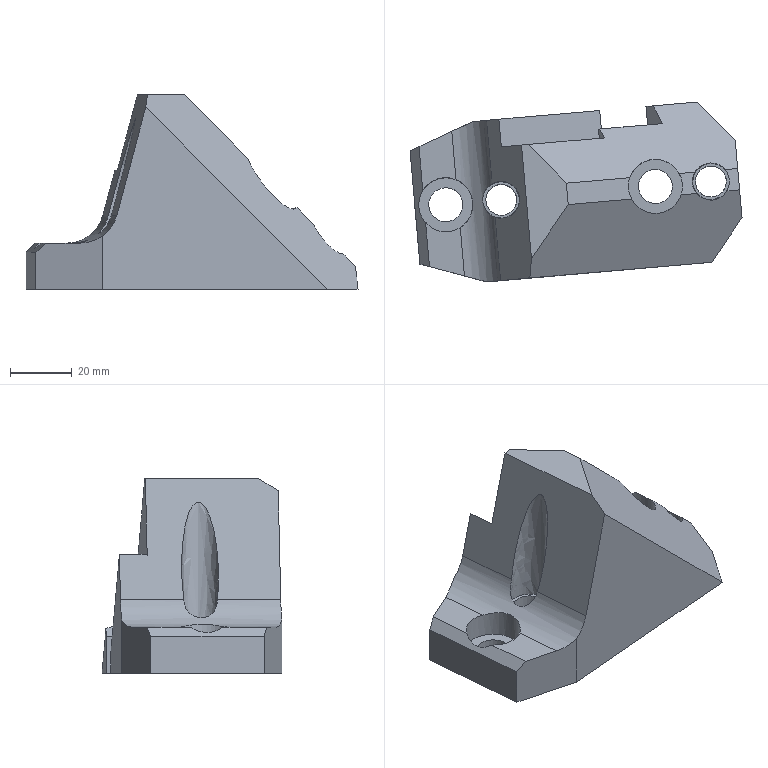Part | NX | features solid 2 | 1 solid | 40 faces | box 107.293 x 58.165 x 63 mm | volume 136956 mm3 | plane 31 | cylinder 7 | spline 2 | commonest cylinder face diameters 10 x2 11 x2 17.5 x2 24 x1
STEP:
#1=CARTESIAN_POINT('',(-404.06,16.31,45.514));
#2=VERTEX_POINT('',#1);
#3=CARTESIAN_POINT('',(-413.818,15.456,55.309));
#4=VERTEX_POINT('',#3);
#5=CARTESIAN_POINT('',(-404.06,16.31,45.514));
#6=CARTESIAN_POINT('',(-404.91,17.317,45.393));
#7=CARTESIAN_POINT('',(-407.23,18.575,46.406));
#8=CARTESIAN_POINT('',(-410.106,18.429,49.198));
#9=CARTESIAN_POINT('',(-412.325,17.358,52.216));
#10=CARTESIAN_POINT('',(-413.406,16.165,54.29));
#11=CARTESIAN_POINT('',(-413.818,15.456,55.309));
#12=B_SPLINE_CURVE_WITH_KNOTS('',3,(#5,#6,#7,#8,#9,#10,#11),.UNSPECIFIED.,.F.,.F.,(4,1,1,1,4),(-0.007434,-0.003558,0.0003178,0.004194,0.00807),.UNSPECIFIED.);
#13=EDGE_CURVE('',#2,#4,#12,.T.);
#14=ORIENTED_EDGE('',*,*,#13,.F.);
#15=CARTESIAN_POINT('',(-399.975,16.667,41.413));
#16=VERTEX_POINT('',#15);
#17=CARTESIAN_POINT('',(-490.277,8.767,132.06));
#18=DIRECTION('',(0.7044,0.06163,-0.7071));
#19=VECTOR('',#18,1000.);
#20=LINE('',#17,#19);
#21=EDGE_CURVE('',#2,#16,#20,.T.);
#22=ORIENTED_EDGE('',*,*,#21,.T.);
#23=CARTESIAN_POINT('',(-400.766,25.712,34.));
#24=VERTEX_POINT('',#23);
#25=CARTESIAN_POINT('',(-397.614,-10.317,63.53));
#26=DIRECTION('',(0.06751,-0.7716,0.6325));
#27=VECTOR('',#26,1000.);
#28=LINE('',#25,#27);
#29=EDGE_CURVE('',#24,#16,#28,.T.);
#30=ORIENTED_EDGE('',*,*,#29,.F.);
#31=CARTESIAN_POINT('',(-412.885,38.16,34.));
#32=VERTEX_POINT('',#31);
#33=CARTESIAN_POINT('',(-451.45,77.774,34.));
#34=DIRECTION('',(-0.6976,0.7165,0.));
#35=VECTOR('',#34,1000.);
#36=LINE('',#33,#35);
#37=EDGE_CURVE('',#24,#32,#36,.T.);
#38=ORIENTED_EDGE('',*,*,#37,.T.);
#39=CARTESIAN_POINT('',(-427.238,36.904,48.408));
#40=VERTEX_POINT('',#39);
#41=CARTESIAN_POINT('',(-501.407,30.415,122.86));
#42=DIRECTION('',(0.7044,0.06163,-0.7071));
#43=VECTOR('',#42,1000.);
#44=LINE('',#41,#43);
#45=EDGE_CURVE('',#40,#32,#44,.T.);
#46=ORIENTED_EDGE('',*,*,#45,.F.);
#47=CARTESIAN_POINT('',(-424.275,31.141,50.857));
#48=VERTEX_POINT('',#47);
#49=CARTESIAN_POINT('',(-426.8,36.054,48.769));
#50=DIRECTION('',(0.4277,-0.8319,0.3536));
#51=VECTOR('',#50,1000.);
#52=LINE('',#49,#51);
#53=EDGE_CURVE('',#40,#48,#52,.T.);
#54=ORIENTED_EDGE('',*,*,#53,.T.);
#55=CARTESIAN_POINT('',(-444.558,29.366,71.219));
#56=VERTEX_POINT('',#55);
#57=CARTESIAN_POINT('',(-498.443,24.652,125.31));
#58=DIRECTION('',(-0.7044,-0.06163,0.7071));
#59=VECTOR('',#58,1000.);
#60=LINE('',#57,#59);
#61=EDGE_CURVE('',#48,#56,#60,.T.);
#62=ORIENTED_EDGE('',*,*,#61,.T.);
#63=CARTESIAN_POINT('',(-443.077,26.484,72.444));
#64=VERTEX_POINT('',#63);
#65=CARTESIAN_POINT('',(-447.084,34.279,69.131));
#66=DIRECTION('',(0.4277,-0.8319,0.3536));
#67=VECTOR('',#66,1000.);
#68=LINE('',#65,#67);
#69=EDGE_CURVE('',#56,#64,#68,.T.);
#70=ORIENTED_EDGE('',*,*,#69,.T.);
#71=CARTESIAN_POINT('',(-467.54,24.344,97.));
#72=VERTEX_POINT('',#71);
#73=CARTESIAN_POINT('',(-496.962,21.77,126.534));
#74=DIRECTION('',(0.7044,0.06163,-0.7071));
#75=VECTOR('',#74,1000.);
#76=LINE('',#73,#75);
#77=EDGE_CURVE('',#72,#64,#76,.T.);
#78=ORIENTED_EDGE('',*,*,#77,.F.);
#79=CARTESIAN_POINT('',(-455.35,11.823,97.));
#80=VERTEX_POINT('',#79);
#81=CARTESIAN_POINT('',(-486.416,43.733,97.));
#82=DIRECTION('',(-0.6976,0.7165,0.));
#83=VECTOR('',#82,1000.);
#84=LINE('',#81,#83);
#85=EDGE_CURVE('',#80,#72,#84,.T.);
#86=ORIENTED_EDGE('',*,*,#85,.F.);
#87=CARTESIAN_POINT('',(-434.875,13.614,76.447));
#88=VERTEX_POINT('',#87);
#89=CARTESIAN_POINT('',(-490.277,8.767,132.06));
#90=DIRECTION('',(0.7044,0.06163,-0.7071));
#91=VECTOR('',#90,1000.);
#92=LINE('',#89,#91);
#93=EDGE_CURVE('',#80,#88,#92,.T.);
#94=ORIENTED_EDGE('',*,*,#93,.T.);
#95=CARTESIAN_POINT('',(-418.866,15.015,60.376));
#96=VERTEX_POINT('',#95);
#97=CARTESIAN_POINT('',(-426.569,10.863,71.24));
#98=DIRECTION('',(-0.5665,-0.5515,-0.6124));
#99=DIRECTION('',(0.4388,0.4272,-0.7906));
#100=AXIS2_PLACEMENT_3D('',#97,#98,#99);
#101=ELLIPSE('',#100,14.289,8.75);
#102=EDGE_CURVE('',#96,#88,#101,.F.);
#103=ORIENTED_EDGE('',*,*,#102,.F.);
#104=CARTESIAN_POINT('',(-490.277,8.767,132.06));
#105=DIRECTION('',(0.7044,0.06163,-0.7071));
#106=VECTOR('',#105,1000.);
#107=LINE('',#104,#106);
#108=EDGE_CURVE('',#96,#4,#107,.T.);
#109=ORIENTED_EDGE('',*,*,#108,.T.);
#110=EDGE_LOOP('',(#14,#22,#30,#38,#46,#54,#62,#70,#78,#86,#94,#103,#109));
#111=FACE_BOUND('',#110,.T.);
#112=CARTESIAN_POINT('',(-500.969,29.565,123.222));
#113=DIRECTION('',(-0.5665,-0.5515,-0.6124));
#114=DIRECTION('',(-0.7044,-0.06163,0.7071));
#115=AXIS2_PLACEMENT_3D('',#112,#113,#114);
#116=PLANE('',#115);
#117=ADVANCED_FACE('',(#111),#116,.F.);
#118=CARTESIAN_POINT('',(-403.457,9.408,45.514));
#119=VERTEX_POINT('',#118);
#120=CARTESIAN_POINT('',(-399.371,9.766,41.413));
#121=VERTEX_POINT('',#120);
#122=CARTESIAN_POINT('',(-489.673,1.865,132.06));
#123=DIRECTION('',(0.7044,0.06163,-0.7071));
#124=VECTOR('',#123,1000.);
#125=LINE('',#122,#124);
#126=EDGE_CURVE('',#119,#121,#125,.T.);
#127=ORIENTED_EDGE('',*,*,#126,.F.);
#128=CARTESIAN_POINT('',(-413.214,8.555,55.309));
#129=VERTEX_POINT('',#128);
#130=CARTESIAN_POINT('',(-413.214,8.555,55.309));
#131=CARTESIAN_POINT('',(-412.685,7.928,54.289));
#132=CARTESIAN_POINT('',(-411.436,6.953,52.248));
#133=CARTESIAN_POINT('',(-409.038,6.268,49.191));
#134=CARTESIAN_POINT('',(-406.185,6.627,46.407));
#135=CARTESIAN_POINT('',(-404.117,8.271,45.394));
#136=CARTESIAN_POINT('',(-403.457,9.408,45.514));
#137=B_SPLINE_CURVE_WITH_KNOTS('',3,(#130,#131,#132,#133,#134,#135,#136),.UNSPECIFIED.,.F.,.F.,(4,1,1,1,4),(0.,0.003871,0.007742,0.01161,0.01548),.UNSPECIFIED.);
#138=EDGE_CURVE('',#129,#119,#137,.T.);
#139=ORIENTED_EDGE('',*,*,#138,.F.);
#140=CARTESIAN_POINT('',(-418.262,8.113,60.376));
#141=VERTEX_POINT('',#140);
#142=CARTESIAN_POINT('',(-489.673,1.865,132.06));
#143=DIRECTION('',(0.7044,0.06163,-0.7071));
#144=VECTOR('',#143,1000.);
#145=LINE('',#142,#144);
#146=EDGE_CURVE('',#141,#129,#145,.T.);
#147=ORIENTED_EDGE('',*,*,#146,.F.);
#148=CARTESIAN_POINT('',(-434.271,6.712,76.447));
#149=VERTEX_POINT('',#148);
#150=CARTESIAN_POINT('',(-426.569,10.863,71.24));
#151=DIRECTION('',(-0.6536,0.4447,-0.6124));
#152=DIRECTION('',(0.5063,-0.3445,-0.7906));
#153=AXIS2_PLACEMENT_3D('',#150,#151,#152);
#154=ELLIPSE('',#153,14.289,8.75);
#155=EDGE_CURVE('',#149,#141,#154,.F.);
#156=ORIENTED_EDGE('',*,*,#155,.F.);
#157=CARTESIAN_POINT('',(-454.746,4.921,97.));
#158=VERTEX_POINT('',#157);
#159=CARTESIAN_POINT('',(-489.673,1.865,132.06));
#160=DIRECTION('',(0.7044,0.06163,-0.7071));
#161=VECTOR('',#160,1000.);
#162=LINE('',#159,#161);
#163=EDGE_CURVE('',#158,#149,#162,.T.);
#164=ORIENTED_EDGE('',*,*,#163,.F.);
#165=CARTESIAN_POINT('',(-466.613,-12.52,97.));
#166=VERTEX_POINT('',#165);
#167=CARTESIAN_POINT('',(-467.532,-13.87,97.));
#168=DIRECTION('',(0.5625,0.8268,0.));
#169=VECTOR('',#168,1000.);
#170=LINE('',#167,#169);
#171=EDGE_CURVE('',#166,#158,#170,.T.);
#172=ORIENTED_EDGE('',*,*,#171,.F.);
#173=CARTESIAN_POINT('',(-467.138,-18.785,93.01));
#174=VERTEX_POINT('',#173);
#175=CARTESIAN_POINT('',(-464.592,11.602,112.36));
#176=DIRECTION('',(0.0705,0.8414,0.5358));
#177=VECTOR('',#176,1000.);
#178=LINE('',#175,#177);
#179=EDGE_CURVE('',#174,#166,#178,.T.);
#180=ORIENTED_EDGE('',*,*,#179,.F.);
#181=CARTESIAN_POINT('',(-408.352,-13.642,34.));
#182=VERTEX_POINT('',#181);
#183=CARTESIAN_POINT('',(-496.874,-21.387,122.86));
#184=DIRECTION('',(0.7044,0.06163,-0.7071));
#185=VECTOR('',#184,1000.);
#186=LINE('',#183,#185);
#187=EDGE_CURVE('',#174,#182,#186,.T.);
#188=ORIENTED_EDGE('',*,*,#187,.T.);
#189=CARTESIAN_POINT('',(-398.58,0.7211,34.));
#190=VERTEX_POINT('',#189);
#191=CARTESIAN_POINT('',(-427.185,-41.321,34.));
#192=DIRECTION('',(0.5625,0.8268,0.));
#193=VECTOR('',#192,1000.);
#194=LINE('',#191,#193);
#195=EDGE_CURVE('',#182,#190,#194,.T.);
#196=ORIENTED_EDGE('',*,*,#195,.T.);
#197=CARTESIAN_POINT('',(-403.204,53.577,77.322));
#198=DIRECTION('',(0.06751,-0.7716,-0.6325));
#199=VECTOR('',#198,1000.);
#200=LINE('',#197,#199);
#201=EDGE_CURVE('',#121,#190,#200,.T.);
#202=ORIENTED_EDGE('',*,*,#201,.F.);
#203=EDGE_LOOP('',(#127,#139,#147,#156,#164,#172,#180,#188,#196,#202));
#204=FACE_BOUND('',#203,.T.);
#205=CARTESIAN_POINT('',(-489.845,1.312,131.842));
#206=DIRECTION('',(-0.6536,0.4447,-0.6124));
#207=DIRECTION('',(-0.7044,-0.06163,0.7071));
#208=AXIS2_PLACEMENT_3D('',#205,#206,#207);
#209=PLANE('',#208);
#210=ADVANCED_FACE('',(#204),#209,.F.);
#211=CARTESIAN_POINT('',(-403.457,9.408,45.514));
#212=CARTESIAN_POINT('',(-402.887,10.388,44.862));
#213=CARTESIAN_POINT('',(-402.211,12.984,43.962));
#214=CARTESIAN_POINT('',(-403.328,15.443,44.861));
#215=CARTESIAN_POINT('',(-404.06,16.31,45.514));
#216=B_SPLINE_CURVE_WITH_KNOTS('',3,(#211,#212,#213,#214,#215),.UNSPECIFIED.,.F.,.F.,(4,1,4),(0.,0.003881,0.007763),.UNSPECIFIED.);
#217=EDGE_CURVE('',#119,#2,#216,.T.);
#218=ORIENTED_EDGE('',*,*,#217,.F.);
#219=ORIENTED_EDGE('',*,*,#126,.T.);
#220=CARTESIAN_POINT('',(-399.371,9.766,41.413));
#221=DIRECTION('',(0.08716,-0.9962,0.));
#222=VECTOR('',#221,1000.);
#223=LINE('',#220,#222);
#224=EDGE_CURVE('',#16,#121,#223,.T.);
#225=ORIENTED_EDGE('',*,*,#224,.F.);
#226=ORIENTED_EDGE('',*,*,#21,.F.);
#227=EDGE_LOOP('',(#218,#219,#225,#226));
#228=FACE_BOUND('',#227,.T.);
#229=CARTESIAN_POINT('',(-489.673,1.865,132.06));
#230=DIRECTION('',(-0.7044,-0.06163,-0.7071));
#231=DIRECTION('',(-0.7044,-0.06163,0.7071));
#232=AXIS2_PLACEMENT_3D('',#229,#230,#231);
#233=PLANE('',#232);
#234=ADVANCED_FACE('',(#228),#233,.F.);
#235=CARTESIAN_POINT('',(-476.512,-19.605,57.892));
#236=VERTEX_POINT('',#235);
#237=CARTESIAN_POINT('',(-478.299,0.8249,57.892));
#238=VERTEX_POINT('',#237);
#239=CARTESIAN_POINT('',(-476.512,-19.605,57.892));
#240=DIRECTION('',(-0.08716,0.9962,0.));
#241=VECTOR('',#240,1000.);
#242=LINE('',#239,#241);
#243=EDGE_CURVE('',#236,#238,#242,.T.);
#244=ORIENTED_EDGE('',*,*,#243,.T.);
#245=CARTESIAN_POINT('',(-479.257,11.767,57.892));
#246=VERTEX_POINT('',#245);
#247=CARTESIAN_POINT('',(-478.299,0.8249,57.892));
#248=CARTESIAN_POINT('',(-478.516,0.8982,57.109));
#249=CARTESIAN_POINT('',(-479.104,1.119,55.621));
#250=CARTESIAN_POINT('',(-480.41,1.933,53.674));
#251=CARTESIAN_POINT('',(-481.783,3.581,52.36));
#252=CARTESIAN_POINT('',(-482.532,5.948,51.903));
#253=CARTESIAN_POINT('',(-482.215,8.435,52.352));
#254=CARTESIAN_POINT('',(-481.151,10.297,53.663));
#255=CARTESIAN_POINT('',(-480.008,11.331,55.597));
#256=CARTESIAN_POINT('',(-479.458,11.656,57.107));
#257=CARTESIAN_POINT('',(-479.257,11.767,57.892));
#258=B_SPLINE_CURVE_WITH_KNOTS('',3,(#247,#248,#249,#250,#251,#252,#253,#254,#255,#256,#257),.UNSPECIFIED.,.F.,.F.,(4,1,1,1,1,1,1,1,4),(0.,0.002417,0.004835,0.007252,0.009669,0.01209,0.0145,0.01692,0.01934),.UNSPECIFIED.);
#259=EDGE_CURVE('',#238,#246,#258,.T.);
#260=ORIENTED_EDGE('',*,*,#259,.T.);
#261=CARTESIAN_POINT('',(-481.044,32.197,57.892));
#262=VERTEX_POINT('',#261);
#263=CARTESIAN_POINT('',(-476.512,-19.605,57.892));
#264=DIRECTION('',(-0.08716,0.9962,0.));
#265=VECTOR('',#264,1000.);
#266=LINE('',#263,#265);
#267=EDGE_CURVE('',#246,#262,#266,.T.);
#268=ORIENTED_EDGE('',*,*,#267,.T.);
#269=CARTESIAN_POINT('',(-485.618,31.797,51.251));
#270=VERTEX_POINT('',#269);
#271=CARTESIAN_POINT('',(-492.591,31.187,60.998));
#272=DIRECTION('',(0.08716,-0.9962,0.));
#273=DIRECTION('',(0.9962,0.08716,0.));
#274=AXIS2_PLACEMENT_3D('',#271,#272,#273);
#275=CIRCLE('',#274,12.);
#276=EDGE_CURVE('',#270,#262,#275,.T.);
#277=ORIENTED_EDGE('',*,*,#276,.F.);
#278=CARTESIAN_POINT('',(-492.369,28.648,48.998));
#279=VERTEX_POINT('',#278);
#280=CARTESIAN_POINT('',(-492.369,28.648,60.998));
#281=DIRECTION('',(0.4226,-0.9063,0.));
#282=DIRECTION('',(0.9063,0.4226,0.));
#283=AXIS2_PLACEMENT_3D('',#280,#281,#282);
#284=ELLIPSE('',#283,12.77,12.);
#285=EDGE_CURVE('',#279,#270,#284,.T.);
#286=ORIENTED_EDGE('',*,*,#285,.F.);
#287=CARTESIAN_POINT('',(-491.003,13.038,48.998));
#288=VERTEX_POINT('',#287);
#289=CARTESIAN_POINT('',(-488.059,-20.616,48.998));
#290=DIRECTION('',(-0.08716,0.9962,0.));
#291=VECTOR('',#290,1000.);
#292=LINE('',#289,#291);
#293=EDGE_CURVE('',#288,#279,#292,.T.);
#294=ORIENTED_EDGE('',*,*,#293,.F.);
#295=CARTESIAN_POINT('',(-489.647,-2.467,48.998));
#296=VERTEX_POINT('',#295);
#297=CARTESIAN_POINT('',(-491.003,13.038,48.998));
#298=CARTESIAN_POINT('',(-489.499,12.424,48.998));
#299=CARTESIAN_POINT('',(-486.924,10.407,49.531));
#300=CARTESIAN_POINT('',(-485.14,5.744,50.201));
#301=CARTESIAN_POINT('',(-486.079,0.845,49.533));
#302=CARTESIAN_POINT('',(-488.272,-1.601,48.998));
#303=CARTESIAN_POINT('',(-489.647,-2.467,48.998));
#304=B_SPLINE_CURVE_WITH_KNOTS('',3,(#297,#298,#299,#300,#301,#302,#303),.UNSPECIFIED.,.F.,.F.,(4,1,1,1,4),(0.,0.004797,0.009594,0.01439,0.01919),.UNSPECIFIED.);
#305=EDGE_CURVE('',#288,#296,#304,.T.);
#306=ORIENTED_EDGE('',*,*,#305,.T.);
#307=CARTESIAN_POINT('',(-488.281,-18.077,48.998));
#308=VERTEX_POINT('',#307);
#309=CARTESIAN_POINT('',(-488.059,-20.616,48.998));
#310=DIRECTION('',(-0.08716,0.9962,0.));
#311=VECTOR('',#310,1000.);
#312=LINE('',#309,#311);
#313=EDGE_CURVE('',#308,#296,#312,.T.);
#314=ORIENTED_EDGE('',*,*,#313,.F.);
#315=CARTESIAN_POINT('',(-481.086,-20.005,51.251));
#316=VERTEX_POINT('',#315);
#317=CARTESIAN_POINT('',(-488.281,-18.077,60.998));
#318=DIRECTION('',(-0.2588,-0.9659,0.));
#319=DIRECTION('',(-0.9659,0.2588,0.));
#320=AXIS2_PLACEMENT_3D('',#317,#318,#319);
#321=ELLIPSE('',#320,12.77,12.);
#322=EDGE_CURVE('',#308,#316,#321,.T.);
#323=ORIENTED_EDGE('',*,*,#322,.T.);
#324=CARTESIAN_POINT('',(-488.059,-20.616,60.998));
#325=DIRECTION('',(0.08716,-0.9962,0.));
#326=DIRECTION('',(0.9962,0.08716,0.));
#327=AXIS2_PLACEMENT_3D('',#324,#325,#326);
#328=CIRCLE('',#327,12.);
#329=EDGE_CURVE('',#316,#236,#328,.T.);
#330=ORIENTED_EDGE('',*,*,#329,.T.);
#331=EDGE_LOOP('',(#244,#260,#268,#277,#286,#294,#306,#314,#323,#330));
#332=FACE_BOUND('',#331,.T.);
#333=CARTESIAN_POINT('',(-488.059,-20.616,60.998));
#334=DIRECTION('',(-0.08716,0.9962,0.));
#335=DIRECTION('',(0.,0.,1.));
#336=AXIS2_PLACEMENT_3D('',#333,#334,#335);
#337=CYLINDRICAL_SURFACE('',#336,12.);
#338=ADVANCED_FACE('',(#332),#337,.F.);
#339=ORIENTED_EDGE('',*,*,#267,.F.);
#340=CARTESIAN_POINT('',(-479.257,11.767,57.892));
#341=CARTESIAN_POINT('',(-478.55,12.153,60.646));
#342=CARTESIAN_POINT('',(-477.466,12.487,64.785));
#343=CARTESIAN_POINT('',(-475.979,12.526,70.325));
#344=CARTESIAN_POINT('',(-474.849,12.343,74.467));
#345=CARTESIAN_POINT('',(-473.705,11.924,78.582));
#346=CARTESIAN_POINT('',(-472.736,11.321,81.991));
#347=CARTESIAN_POINT('',(-471.957,10.591,84.648));
#348=CARTESIAN_POINT('',(-471.37,9.857,86.591));
#349=CARTESIAN_POINT('',(-470.888,8.997,88.106));
#350=CARTESIAN_POINT('',(-470.535,7.975,89.085));
#351=CARTESIAN_POINT('',(-470.354,6.887,89.402));
#352=CARTESIAN_POINT('',(-470.393,5.853,88.921));
#353=CARTESIAN_POINT('',(-470.583,4.853,87.892));
#354=CARTESIAN_POINT('',(-470.917,3.963,86.359));
#355=CARTESIAN_POINT('',(-471.368,3.169,84.423));
#356=CARTESIAN_POINT('',(-472.012,2.337,81.76));
#357=CARTESIAN_POINT('',(-472.85,1.604,78.405));
#358=CARTESIAN_POINT('',(-473.893,1.008,74.333));
#359=CARTESIAN_POINT('',(-474.965,0.64,70.228));
#360=CARTESIAN_POINT('',(-476.425,0.4275,64.73));
#361=CARTESIAN_POINT('',(-477.542,0.569,60.625));
#362=CARTESIAN_POINT('',(-478.299,0.8249,57.892));
#363=B_SPLINE_CURVE_WITH_KNOTS('',3,(#340,#341,#342,#343,#344,#345,#346,#347,#348,#349,#350,#351,#352,#353,#354,#355,#356,#357,#358,#359,#360,#361,#362),.UNSPECIFIED.,.F.,.F.,(4,1,1,1,1,1,1,1,1,1,1,1,1,1,1,1,1,1,1,1,4),(0.,0.008585,0.01288,0.01717,0.02146,0.02575,0.0279,0.03005,0.03219,0.03327,0.03434,0.03541,0.03649,0.03863,0.04078,0.04292,0.04722,0.05151,0.0558,0.06009,0.06868),.UNSPECIFIED.);
#364=EDGE_CURVE('',#246,#238,#363,.T.);
#365=ORIENTED_EDGE('',*,*,#364,.T.);
#366=ORIENTED_EDGE('',*,*,#243,.F.);
#367=CARTESIAN_POINT('',(-476.512,-19.605,57.892));
#368=DIRECTION('',(0.2578,0.02256,0.9659));
#369=VECTOR('',#368,1000.);
#370=LINE('',#367,#369);
#371=EDGE_CURVE('',#236,#174,#370,.T.);
#372=ORIENTED_EDGE('',*,*,#371,.T.);
#373=ORIENTED_EDGE('',*,*,#179,.T.);
#374=CARTESIAN_POINT('',(-469.821,24.144,97.));
#375=VERTEX_POINT('',#374);
#376=CARTESIAN_POINT('',(-466.073,-18.692,97.));
#377=DIRECTION('',(-0.08716,0.9962,0.));
#378=VECTOR('',#377,1000.);
#379=LINE('',#376,#378);
#380=EDGE_CURVE('',#166,#375,#379,.T.);
#381=ORIENTED_EDGE('',*,*,#380,.T.);
#382=CARTESIAN_POINT('',(-476.359,23.572,72.504));
#383=VERTEX_POINT('',#382);
#384=CARTESIAN_POINT('',(-480.26,23.231,57.892));
#385=DIRECTION('',(0.2578,0.02256,0.9659));
#386=VECTOR('',#385,1000.);
#387=LINE('',#384,#386);
#388=EDGE_CURVE('',#383,#375,#387,.T.);
#389=ORIENTED_EDGE('',*,*,#388,.F.);
#390=CARTESIAN_POINT('',(-477.144,32.538,72.504));
#391=VERTEX_POINT('',#390);
#392=CARTESIAN_POINT('',(-472.612,-19.264,72.504));
#393=DIRECTION('',(0.08716,-0.9962,0.));
#394=VECTOR('',#393,1000.);
#395=LINE('',#392,#394);
#396=EDGE_CURVE('',#391,#383,#395,.T.);
#397=ORIENTED_EDGE('',*,*,#396,.F.);
#398=CARTESIAN_POINT('',(-481.044,32.197,57.892));
#399=DIRECTION('',(0.2578,0.02256,0.9659));
#400=VECTOR('',#399,1000.);
#401=LINE('',#398,#400);
#402=EDGE_CURVE('',#262,#391,#401,.T.);
#403=ORIENTED_EDGE('',*,*,#402,.F.);
#404=EDGE_LOOP('',(#339,#365,#366,#372,#373,#381,#389,#397,#403));
#405=FACE_BOUND('',#404,.T.);
#406=CARTESIAN_POINT('',(-476.512,-19.605,57.892));
#407=DIRECTION('',(-0.9623,-0.08419,0.2588));
#408=DIRECTION('',(0.2578,0.02256,0.9659));
#409=AXIS2_PLACEMENT_3D('',#406,#407,#408);
#410=PLANE('',#409);
#411=ADVANCED_FACE('',(#405),#410,.T.);
#412=CARTESIAN_POINT('',(-413.818,15.456,55.309));
#413=CARTESIAN_POINT('',(-414.387,14.476,55.961));
#414=CARTESIAN_POINT('',(-415.063,11.88,56.861));
#415=CARTESIAN_POINT('',(-413.946,9.422,55.962));
#416=CARTESIAN_POINT('',(-413.214,8.555,55.309));
#417=B_SPLINE_CURVE_WITH_KNOTS('',3,(#412,#413,#414,#415,#416),.UNSPECIFIED.,.F.,.F.,(4,1,4),(0.,0.003881,0.007763),.UNSPECIFIED.);
#418=EDGE_CURVE('',#4,#129,#417,.T.);
#419=ORIENTED_EDGE('',*,*,#418,.F.);
#420=ORIENTED_EDGE('',*,*,#108,.F.);
#421=CARTESIAN_POINT('',(-426.569,10.863,68.411));
#422=DIRECTION('',(-0.7044,-0.06163,-0.7071));
#423=DIRECTION('',(0.7044,0.06163,-0.7071));
#424=AXIS2_PLACEMENT_3D('',#421,#422,#423);
#425=ELLIPSE('',#424,12.374,8.75);
#426=EDGE_CURVE('',#141,#96,#425,.F.);
#427=ORIENTED_EDGE('',*,*,#426,.F.);
#428=ORIENTED_EDGE('',*,*,#146,.T.);
#429=EDGE_LOOP('',(#419,#420,#427,#428));
#430=FACE_BOUND('',#429,.T.);
#431=CARTESIAN_POINT('',(-489.673,1.865,132.06));
#432=DIRECTION('',(-0.7044,-0.06163,-0.7071));
#433=DIRECTION('',(-0.7044,-0.06163,0.7071));
#434=AXIS2_PLACEMENT_3D('',#431,#432,#433);
#435=PLANE('',#434);
#436=ADVANCED_FACE('',(#430),#435,.F.);
#437=ORIENTED_EDGE('',*,*,#313,.T.);
#438=CARTESIAN_POINT('',(-500.826,-0.9033,48.998));
#439=VERTEX_POINT('',#438);
#440=CARTESIAN_POINT('',(-494.31,4.937,48.998));
#441=DIRECTION('',(0.,0.,1.));
#442=DIRECTION('',(0.9962,0.08716,0.));
#443=AXIS2_PLACEMENT_3D('',#440,#441,#442);
#444=CIRCLE('',#443,8.75);
#445=EDGE_CURVE('',#296,#439,#444,.F.);
#446=ORIENTED_EDGE('',*,*,#445,.T.);
#447=CARTESIAN_POINT('',(-499.588,-15.048,48.998));
#448=VERTEX_POINT('',#447);
#449=CARTESIAN_POINT('',(-499.017,-21.574,48.998));
#450=DIRECTION('',(-0.08716,0.9962,0.));
#451=VECTOR('',#450,1000.);
#452=LINE('',#449,#451);
#453=EDGE_CURVE('',#448,#439,#452,.T.);
#454=ORIENTED_EDGE('',*,*,#453,.F.);
#455=CARTESIAN_POINT('',(-497.424,-15.628,48.998));
#456=DIRECTION('',(0.9659,-0.2588,0.));
#457=VECTOR('',#456,1000.);
#458=LINE('',#455,#457);
#459=EDGE_CURVE('',#448,#308,#458,.T.);
#460=ORIENTED_EDGE('',*,*,#459,.T.);
#461=EDGE_LOOP('',(#437,#446,#454,#460));
#462=FACE_BOUND('',#461,.T.);
#463=CARTESIAN_POINT('',(-499.017,-21.574,48.998));
#464=DIRECTION('',(0.,0.,1.));
#465=DIRECTION('',(0.9962,0.08716,0.));
#466=AXIS2_PLACEMENT_3D('',#463,#464,#465);
#467=PLANE('',#466);
#468=ADVANCED_FACE('',(#462),#467,.T.);
#469=CARTESIAN_POINT('',(-501.741,9.557,48.998));
#470=VERTEX_POINT('',#469);
#471=CARTESIAN_POINT('',(-502.978,23.701,48.998));
#472=VERTEX_POINT('',#471);
#473=CARTESIAN_POINT('',(-499.017,-21.574,48.998));
#474=DIRECTION('',(-0.08716,0.9962,0.));
#475=VECTOR('',#474,1000.);
#476=LINE('',#473,#475);
#477=EDGE_CURVE('',#470,#472,#476,.T.);
#478=ORIENTED_EDGE('',*,*,#477,.F.);
#479=CARTESIAN_POINT('',(-494.31,4.937,48.998));
#480=DIRECTION('',(0.,0.,1.));
#481=DIRECTION('',(0.9962,0.08716,0.));
#482=AXIS2_PLACEMENT_3D('',#479,#480,#481);
#483=CIRCLE('',#482,8.75);
#484=EDGE_CURVE('',#470,#288,#483,.F.);
#485=ORIENTED_EDGE('',*,*,#484,.T.);
#486=ORIENTED_EDGE('',*,*,#293,.T.);
#487=CARTESIAN_POINT('',(-517.066,17.132,48.998));
#488=DIRECTION('',(0.9063,0.4226,0.));
#489=VECTOR('',#488,1000.);
#490=LINE('',#487,#489);
#491=EDGE_CURVE('',#472,#279,#490,.T.);
#492=ORIENTED_EDGE('',*,*,#491,.F.);
#493=EDGE_LOOP('',(#478,#485,#486,#492));
#494=FACE_BOUND('',#493,.T.);
#495=CARTESIAN_POINT('',(-499.017,-21.574,48.998));
#496=DIRECTION('',(0.,0.,1.));
#497=DIRECTION('',(0.9962,0.08716,0.));
#498=AXIS2_PLACEMENT_3D('',#495,#496,#497);
#499=PLANE('',#498);
#500=ADVANCED_FACE('',(#494),#499,.T.);
#501=CARTESIAN_POINT('',(-494.31,4.937,55.998));
#502=DIRECTION('',(0.7044,0.06163,-0.7071));
#503=DIRECTION('',(-0.7044,-0.06163,-0.7071));
#504=AXIS2_PLACEMENT_3D('',#501,#502,#503);
#505=ELLIPSE('',#504,12.374,8.75);
#506=EDGE_CURVE('',#470,#439,#505,.F.);
#507=ORIENTED_EDGE('',*,*,#506,.F.);
#508=ORIENTED_EDGE('',*,*,#477,.T.);
#509=CARTESIAN_POINT('',(-505.873,22.351,45.996));
#510=VERTEX_POINT('',#509);
#511=CARTESIAN_POINT('',(-510.46,20.213,41.241));
#512=DIRECTION('',(-0.6605,-0.308,-0.6848));
#513=VECTOR('',#512,1000.);
#514=LINE('',#511,#513);
#515=EDGE_CURVE('',#472,#510,#514,.T.);
#516=ORIENTED_EDGE('',*,*,#515,.T.);
#517=CARTESIAN_POINT('',(-502.673,-14.221,45.996));
#518=VERTEX_POINT('',#517);
#519=CARTESIAN_POINT('',(-502.007,-21.836,45.996));
#520=DIRECTION('',(-0.08716,0.9962,0.));
#521=VECTOR('',#520,1000.);
#522=LINE('',#519,#521);
#523=EDGE_CURVE('',#518,#510,#522,.T.);
#524=ORIENTED_EDGE('',*,*,#523,.F.);
#525=CARTESIAN_POINT('',(-498.439,-15.356,50.116));
#526=DIRECTION('',(-0.7039,0.1886,-0.6848));
#527=VECTOR('',#526,1000.);
#528=LINE('',#525,#527);
#529=EDGE_CURVE('',#448,#518,#528,.T.);
#530=ORIENTED_EDGE('',*,*,#529,.F.);
#531=ORIENTED_EDGE('',*,*,#453,.T.);
#532=EDGE_LOOP('',(#507,#508,#516,#524,#530,#531));
#533=FACE_BOUND('',#532,.T.);
#534=CARTESIAN_POINT('',(-499.017,-21.574,48.998));
#535=DIRECTION('',(0.7044,0.06163,-0.7071));
#536=DIRECTION('',(-0.7044,-0.06163,-0.7071));
#537=AXIS2_PLACEMENT_3D('',#534,#535,#536);
#538=PLANE('',#537);
#539=ADVANCED_FACE('',(#533),#538,.F.);
#540=CARTESIAN_POINT('',(-488.831,5.416,34.));
#541=VERTEX_POINT('',#540);
#542=CARTESIAN_POINT('',(-494.31,4.937,34.));
#543=DIRECTION('',(0.,0.,1.));
#544=DIRECTION('',(0.9962,0.08716,0.));
#545=AXIS2_PLACEMENT_3D('',#542,#543,#544);
#546=CIRCLE('',#545,5.5);
#547=EDGE_CURVE('',#541,#541,#546,.T.);
#548=ORIENTED_EDGE('',*,*,#547,.F.);
#549=EDGE_LOOP('',(#548));
#550=FACE_BOUND('',#549,.T.);
#551=CARTESIAN_POINT('',(-488.831,5.416,40.998));
#552=VERTEX_POINT('',#551);
#553=CARTESIAN_POINT('',(-494.31,4.937,40.998));
#554=DIRECTION('',(0.,0.,1.));
#555=DIRECTION('',(0.9962,0.08716,0.));
#556=AXIS2_PLACEMENT_3D('',#553,#554,#555);
#557=CIRCLE('',#556,5.5);
#558=EDGE_CURVE('',#552,#552,#557,.T.);
#559=ORIENTED_EDGE('',*,*,#558,.T.);
#560=EDGE_LOOP('',(#559));
#561=FACE_BOUND('',#560,.T.);
#562=CARTESIAN_POINT('',(-494.31,4.937,133.998));
#563=DIRECTION('',(0.,0.,-1.));
#564=DIRECTION('',(-0.9962,-0.08716,0.));
#565=AXIS2_PLACEMENT_3D('',#562,#563,#564);
#566=CYLINDRICAL_SURFACE('',#565,5.5);
#567=ADVANCED_FACE('',(#550,#561),#566,.F.);
#568=CARTESIAN_POINT('',(-426.569,10.863,68.411));
#569=DIRECTION('',(-0.7044,-0.06163,-0.7071));
#570=DIRECTION('',(0.7044,0.06163,-0.7071));
#571=AXIS2_PLACEMENT_3D('',#568,#569,#570);
#572=ELLIPSE('',#571,12.374,8.75);
#573=EDGE_CURVE('',#88,#149,#572,.F.);
#574=ORIENTED_EDGE('',*,*,#573,.F.);
#575=ORIENTED_EDGE('',*,*,#93,.F.);
#576=CARTESIAN_POINT('',(-454.746,4.921,97.));
#577=DIRECTION('',(-0.08716,0.9962,0.));
#578=VECTOR('',#577,1000.);
#579=LINE('',#576,#578);
#580=EDGE_CURVE('',#158,#80,#579,.T.);
#581=ORIENTED_EDGE('',*,*,#580,.F.);
#582=ORIENTED_EDGE('',*,*,#163,.T.);
#583=EDGE_LOOP('',(#574,#575,#581,#582));
#584=FACE_BOUND('',#583,.T.);
#585=CARTESIAN_POINT('',(-489.673,1.865,132.06));
#586=DIRECTION('',(-0.7044,-0.06163,-0.7071));
#587=DIRECTION('',(-0.7044,-0.06163,0.7071));
#588=AXIS2_PLACEMENT_3D('',#585,#586,#587);
#589=PLANE('',#588);
#590=ADVANCED_FACE('',(#584),#589,.F.);
#591=CARTESIAN_POINT('',(-421.089,11.343,34.));
#592=VERTEX_POINT('',#591);
#593=CARTESIAN_POINT('',(-426.569,10.863,34.));
#594=DIRECTION('',(0.,0.,1.));
#595=DIRECTION('',(0.9962,0.08716,0.));
#596=AXIS2_PLACEMENT_3D('',#593,#594,#595);
#597=CIRCLE('',#596,5.5);
#598=EDGE_CURVE('',#592,#592,#597,.T.);
#599=ORIENTED_EDGE('',*,*,#598,.F.);
#600=EDGE_LOOP('',(#599));
#601=FACE_BOUND('',#600,.T.);
#602=CARTESIAN_POINT('',(-421.089,11.343,40.998));
#603=VERTEX_POINT('',#602);
#604=CARTESIAN_POINT('',(-426.569,10.863,40.998));
#605=DIRECTION('',(0.,0.,1.));
#606=DIRECTION('',(0.9962,0.08716,0.));
#607=AXIS2_PLACEMENT_3D('',#604,#605,#606);
#608=CIRCLE('',#607,5.5);
#609=EDGE_CURVE('',#603,#603,#608,.T.);
#610=ORIENTED_EDGE('',*,*,#609,.T.);
#611=EDGE_LOOP('',(#610));
#612=FACE_BOUND('',#611,.T.);
#613=CARTESIAN_POINT('',(-426.569,10.863,133.998));
#614=DIRECTION('',(0.,0.,-1.));
#615=DIRECTION('',(-0.9962,-0.08716,0.));
#616=AXIS2_PLACEMENT_3D('',#613,#614,#615);
#617=CYLINDRICAL_SURFACE('',#616,5.5);
#618=ADVANCED_FACE('',(#601,#612),#617,.F.);
#619=CARTESIAN_POINT('',(-471.397,6.941,34.));
#620=VERTEX_POINT('',#619);
#621=CARTESIAN_POINT('',(-476.378,6.506,34.));
#622=DIRECTION('',(0.,0.,1.));
#623=DIRECTION('',(0.9962,0.08716,0.));
#624=AXIS2_PLACEMENT_3D('',#621,#622,#623);
#625=CIRCLE('',#624,5.);
#626=EDGE_CURVE('',#620,#620,#625,.T.);
#627=ORIENTED_EDGE('',*,*,#626,.T.);
#628=EDGE_LOOP('',(#627));
#629=FACE_BOUND('',#628,.T.);
#630=CARTESIAN_POINT('',(-403.656,12.868,34.));
#631=VERTEX_POINT('',#630);
#632=CARTESIAN_POINT('',(-408.637,12.432,34.));
#633=DIRECTION('',(0.,0.,1.));
#634=DIRECTION('',(0.9962,0.08716,0.));
#635=AXIS2_PLACEMENT_3D('',#632,#633,#634);
#636=CIRCLE('',#635,5.);
#637=EDGE_CURVE('',#631,#631,#636,.T.);
#638=ORIENTED_EDGE('',*,*,#637,.T.);
#639=EDGE_LOOP('',(#638));
#640=FACE_BOUND('',#639,.T.);
#641=CARTESIAN_POINT('',(-502.673,-14.221,34.));
#642=VERTEX_POINT('',#641);
#643=CARTESIAN_POINT('',(-481.086,-20.005,34.));
#644=VERTEX_POINT('',#643);
#645=CARTESIAN_POINT('',(-500.147,-14.898,34.));
#646=DIRECTION('',(0.9659,-0.2588,0.));
#647=VECTOR('',#646,1000.);
#648=LINE('',#645,#647);
#649=EDGE_CURVE('',#642,#644,#648,.T.);
#650=ORIENTED_EDGE('',*,*,#649,.F.);
#651=CARTESIAN_POINT('',(-505.873,22.351,34.));
#652=VERTEX_POINT('',#651);
#653=CARTESIAN_POINT('',(-504.36,5.061,34.));
#654=DIRECTION('',(-0.08716,0.9962,0.));
#655=VECTOR('',#654,1000.);
#656=LINE('',#653,#655);
#657=EDGE_CURVE('',#642,#652,#656,.T.);
#658=ORIENTED_EDGE('',*,*,#657,.T.);
#659=CARTESIAN_POINT('',(-485.618,31.797,34.));
#660=VERTEX_POINT('',#659);
#661=CARTESIAN_POINT('',(-519.621,15.941,34.));
#662=DIRECTION('',(0.9063,0.4226,0.));
#663=VECTOR('',#662,1000.);
#664=LINE('',#661,#663);
#665=EDGE_CURVE('',#652,#660,#664,.T.);
#666=ORIENTED_EDGE('',*,*,#665,.T.);
#667=CARTESIAN_POINT('',(-444.565,35.388,34.));
#668=VERTEX_POINT('',#667);
#669=CARTESIAN_POINT('',(-522.539,28.566,34.));
#670=DIRECTION('',(0.9962,0.08716,0.));
#671=VECTOR('',#670,1000.);
#672=LINE('',#669,#671);
#673=EDGE_CURVE('',#660,#668,#672,.T.);
#674=ORIENTED_EDGE('',*,*,#673,.T.);
#675=CARTESIAN_POINT('',(-443.781,26.422,34.));
#676=VERTEX_POINT('',#675);
#677=CARTESIAN_POINT('',(-444.565,35.388,34.));
#678=DIRECTION('',(0.08716,-0.9962,0.));
#679=VECTOR('',#678,1000.);
#680=LINE('',#677,#679);
#681=EDGE_CURVE('',#668,#676,#680,.T.);
#682=ORIENTED_EDGE('',*,*,#681,.T.);
#683=CARTESIAN_POINT('',(-428.838,27.73,34.));
#684=VERTEX_POINT('',#683);
#685=CARTESIAN_POINT('',(-443.781,26.422,34.));
#686=DIRECTION('',(0.9962,0.08716,0.));
#687=VECTOR('',#686,1000.);
#688=LINE('',#685,#687);
#689=EDGE_CURVE('',#676,#684,#688,.T.);
#690=ORIENTED_EDGE('',*,*,#689,.T.);
#691=CARTESIAN_POINT('',(-429.623,36.696,34.));
#692=VERTEX_POINT('',#691);
#693=CARTESIAN_POINT('',(-429.623,36.696,34.));
#694=DIRECTION('',(0.08716,-0.9962,0.));
#695=VECTOR('',#694,1000.);
#696=LINE('',#693,#695);
#697=EDGE_CURVE('',#692,#684,#696,.T.);
#698=ORIENTED_EDGE('',*,*,#697,.F.);
#699=CARTESIAN_POINT('',(-522.539,28.566,34.));
#700=DIRECTION('',(0.9962,0.08716,0.));
#701=VECTOR('',#700,1000.);
#702=LINE('',#699,#701);
#703=EDGE_CURVE('',#692,#32,#702,.T.);
#704=ORIENTED_EDGE('',*,*,#703,.T.);
#705=ORIENTED_EDGE('',*,*,#37,.F.);
#706=CARTESIAN_POINT('',(-397.407,-12.685,34.));
#707=DIRECTION('',(0.08716,-0.9962,0.));
#708=VECTOR('',#707,1000.);
#709=LINE('',#706,#708);
#710=EDGE_CURVE('',#24,#190,#709,.T.);
#711=ORIENTED_EDGE('',*,*,#710,.T.);
#712=ORIENTED_EDGE('',*,*,#195,.F.);
#713=CARTESIAN_POINT('',(-518.007,-23.236,34.));
#714=DIRECTION('',(0.9962,0.08716,0.));
#715=VECTOR('',#714,1000.);
#716=LINE('',#713,#715);
#717=EDGE_CURVE('',#644,#182,#716,.T.);
#718=ORIENTED_EDGE('',*,*,#717,.F.);
#719=EDGE_LOOP('',(#650,#658,#666,#674,#682,#690,#698,#704,#705,#711,#712,#718));
#720=FACE_BOUND('',#719,.T.);
#721=ORIENTED_EDGE('',*,*,#598,.T.);
#722=EDGE_LOOP('',(#721));
#723=FACE_BOUND('',#722,.T.);
#724=ORIENTED_EDGE('',*,*,#547,.T.);
#725=EDGE_LOOP('',(#724));
#726=FACE_BOUND('',#725,.T.);
#727=CARTESIAN_POINT('',(-502.006,-21.836,34.));
#728=DIRECTION('',(0.,0.,1.));
#729=DIRECTION('',(0.08716,-0.9962,0.));
#730=AXIS2_PLACEMENT_3D('',#727,#728,#729);
#731=PLANE('',#730);
#732=ADVANCED_FACE('',(#629,#640,#720,#723,#726),#731,.F.);
#733=CARTESIAN_POINT('',(-481.086,-20.005,101.647));
#734=DIRECTION('',(0.,0.,1.));
#735=VECTOR('',#734,1000.);
#736=LINE('',#733,#735);
#737=EDGE_CURVE('',#644,#316,#736,.T.);
#738=ORIENTED_EDGE('',*,*,#737,.F.);
#739=ORIENTED_EDGE('',*,*,#717,.T.);
#740=ORIENTED_EDGE('',*,*,#187,.F.);
#741=ORIENTED_EDGE('',*,*,#371,.F.);
#742=ORIENTED_EDGE('',*,*,#329,.F.);
#743=EDGE_LOOP('',(#738,#739,#740,#741,#742));
#744=FACE_BOUND('',#743,.T.);
#745=CARTESIAN_POINT('',(-518.007,-23.236,101.647));
#746=DIRECTION('',(-0.08716,0.9962,0.));
#747=DIRECTION('',(0.,0.,1.));
#748=AXIS2_PLACEMENT_3D('',#745,#746,#747);
#749=PLANE('',#748);
#750=ADVANCED_FACE('',(#744),#749,.F.);
#751=ORIENTED_EDGE('',*,*,#657,.F.);
#752=CARTESIAN_POINT('',(-502.673,-14.221,33.998));
#753=DIRECTION('',(0.,0.,1.));
#754=VECTOR('',#753,1000.);
#755=LINE('',#752,#754);
#756=EDGE_CURVE('',#642,#518,#755,.T.);
#757=ORIENTED_EDGE('',*,*,#756,.T.);
#758=ORIENTED_EDGE('',*,*,#523,.T.);
#759=CARTESIAN_POINT('',(-505.873,22.351,33.998));
#760=DIRECTION('',(0.,0.,1.));
#761=VECTOR('',#760,1000.);
#762=LINE('',#759,#761);
#763=EDGE_CURVE('',#652,#510,#762,.T.);
#764=ORIENTED_EDGE('',*,*,#763,.F.);
#765=EDGE_LOOP('',(#751,#757,#758,#764));
#766=FACE_BOUND('',#765,.T.);
#767=CARTESIAN_POINT('',(-504.36,5.061,33.998));
#768=DIRECTION('',(-0.9962,-0.08716,0.));
#769=DIRECTION('',(0.08716,-0.9962,0.));
#770=AXIS2_PLACEMENT_3D('',#767,#768,#769);
#771=PLANE('',#770);
#772=ADVANCED_FACE('',(#766),#771,.T.);
#773=ORIENTED_EDGE('',*,*,#703,.F.);
#774=CARTESIAN_POINT('',(-429.623,36.696,46.014));
#775=VERTEX_POINT('',#774);
#776=CARTESIAN_POINT('',(-429.623,36.696,46.014));
#777=DIRECTION('',(0.,0.,-1.));
#778=VECTOR('',#777,1000.);
#779=LINE('',#776,#778);
#780=EDGE_CURVE('',#775,#692,#779,.T.);
#781=ORIENTED_EDGE('',*,*,#780,.F.);
#782=CARTESIAN_POINT('',(-440.189,35.771,35.407));
#783=DIRECTION('',(0.7044,0.06163,0.7071));
#784=VECTOR('',#783,1000.);
#785=LINE('',#782,#784);
#786=EDGE_CURVE('',#775,#40,#785,.T.);
#787=ORIENTED_EDGE('',*,*,#786,.T.);
#788=ORIENTED_EDGE('',*,*,#45,.T.);
#789=EDGE_LOOP('',(#773,#781,#787,#788));
#790=FACE_BOUND('',#789,.T.);
#791=CARTESIAN_POINT('',(-522.539,28.566,101.647));
#792=DIRECTION('',(-0.08716,0.9962,0.));
#793=DIRECTION('',(0.,0.,1.));
#794=AXIS2_PLACEMENT_3D('',#791,#792,#793);
#795=PLANE('',#794);
#796=ADVANCED_FACE('',(#790),#795,.T.);
#797=ORIENTED_EDGE('',*,*,#786,.F.);
#798=CARTESIAN_POINT('',(-428.838,27.73,46.014));
#799=VERTEX_POINT('',#798);
#800=CARTESIAN_POINT('',(-429.623,36.696,46.014));
#801=DIRECTION('',(0.08716,-0.9962,0.));
#802=VECTOR('',#801,1000.);
#803=LINE('',#800,#802);
#804=EDGE_CURVE('',#775,#799,#803,.T.);
#805=ORIENTED_EDGE('',*,*,#804,.T.);
#806=CARTESIAN_POINT('',(-426.514,27.933,48.347));
#807=VERTEX_POINT('',#806);
#808=CARTESIAN_POINT('',(-439.404,26.805,35.407));
#809=DIRECTION('',(0.7044,0.06163,0.7071));
#810=VECTOR('',#809,1000.);
#811=LINE('',#808,#810);
#812=EDGE_CURVE('',#799,#807,#811,.T.);
#813=ORIENTED_EDGE('',*,*,#812,.T.);
#814=CARTESIAN_POINT('',(-426.775,30.922,48.347));
#815=VERTEX_POINT('',#814);
#816=CARTESIAN_POINT('',(-427.298,36.899,48.347));
#817=DIRECTION('',(0.08716,-0.9962,0.));
#818=VECTOR('',#817,1000.);
#819=LINE('',#816,#818);
#820=EDGE_CURVE('',#815,#807,#819,.T.);
#821=ORIENTED_EDGE('',*,*,#820,.F.);
#822=CARTESIAN_POINT('',(-422.76,31.273,52.378));
#823=DIRECTION('',(-0.7044,-0.06163,-0.7071));
#824=VECTOR('',#823,1000.);
#825=LINE('',#822,#824);
#826=EDGE_CURVE('',#48,#815,#825,.T.);
#827=ORIENTED_EDGE('',*,*,#826,.F.);
#828=ORIENTED_EDGE('',*,*,#53,.F.);
#829=EDGE_LOOP('',(#797,#805,#813,#821,#827,#828));
#830=FACE_BOUND('',#829,.T.);
#831=CARTESIAN_POINT('',(-440.189,35.771,35.407));
#832=DIRECTION('',(-0.7044,-0.06163,0.7071));
#833=DIRECTION('',(0.7044,0.06163,0.7071));
#834=AXIS2_PLACEMENT_3D('',#831,#832,#833);
#835=PLANE('',#834);
#836=ADVANCED_FACE('',(#830),#835,.T.);
#837=CARTESIAN_POINT('',(-444.946,29.332,66.588));
#838=VERTEX_POINT('',#837);
#839=CARTESIAN_POINT('',(-426.775,30.922,48.347));
#840=DIRECTION('',(-0.7044,-0.06163,0.7071));
#841=VECTOR('',#840,1000.);
#842=LINE('',#839,#841);
#843=EDGE_CURVE('',#815,#838,#842,.T.);
#844=ORIENTED_EDGE('',*,*,#843,.T.);
#845=CARTESIAN_POINT('',(-444.946,29.332,70.83));
#846=VERTEX_POINT('',#845);
#847=CARTESIAN_POINT('',(-444.946,29.332,66.588));
#848=DIRECTION('',(0.,0.,1.));
#849=VECTOR('',#848,1000.);
#850=LINE('',#847,#849);
#851=EDGE_CURVE('',#838,#846,#850,.T.);
#852=ORIENTED_EDGE('',*,*,#851,.T.);
#853=CARTESIAN_POINT('',(-449.383,28.944,66.375));
#854=DIRECTION('',(0.7044,0.06163,0.7071));
#855=VECTOR('',#854,1000.);
#856=LINE('',#853,#855);
#857=EDGE_CURVE('',#846,#56,#856,.T.);
#858=ORIENTED_EDGE('',*,*,#857,.T.);
#859=ORIENTED_EDGE('',*,*,#61,.F.);
#860=ORIENTED_EDGE('',*,*,#826,.T.);
#861=EDGE_LOOP('',(#844,#852,#858,#859,#860));
#862=FACE_BOUND('',#861,.T.);
#863=CARTESIAN_POINT('',(-483.195,25.986,100.317));
#864=DIRECTION('',(0.08716,-0.9962,0.));
#865=DIRECTION('',(0.,0.,-1.));
#866=AXIS2_PLACEMENT_3D('',#863,#864,#865);
#867=PLANE('',#866);
#868=ADVANCED_FACE('',(#862),#867,.F.);
#869=ORIENTED_EDGE('',*,*,#857,.F.);
#870=CARTESIAN_POINT('',(-444.684,26.343,70.83));
#871=VERTEX_POINT('',#870);
#872=CARTESIAN_POINT('',(-444.684,26.343,70.83));
#873=DIRECTION('',(0.08716,-0.9962,0.));
#874=VECTOR('',#873,1000.);
#875=LINE('',#872,#874);
#876=EDGE_CURVE('',#846,#871,#875,.T.);
#877=ORIENTED_EDGE('',*,*,#876,.T.);
#878=CARTESIAN_POINT('',(-442.782,26.51,72.739));
#879=DIRECTION('',(-0.7044,-0.06163,-0.7071));
#880=VECTOR('',#879,1000.);
#881=LINE('',#878,#880);
#882=EDGE_CURVE('',#64,#871,#881,.T.);
#883=ORIENTED_EDGE('',*,*,#882,.F.);
#884=ORIENTED_EDGE('',*,*,#69,.F.);
#885=EDGE_LOOP('',(#869,#877,#883,#884));
#886=FACE_BOUND('',#885,.T.);
#887=CARTESIAN_POINT('',(-442.782,26.51,72.739));
#888=DIRECTION('',(0.7044,0.06163,-0.7071));
#889=DIRECTION('',(-0.7044,-0.06163,-0.7071));
#890=AXIS2_PLACEMENT_3D('',#887,#888,#889);
#891=PLANE('',#890);
#892=ADVANCED_FACE('',(#886),#891,.F.);
#893=ORIENTED_EDGE('',*,*,#85,.T.);
#894=CARTESIAN_POINT('',(-469.821,24.144,97.));
#895=DIRECTION('',(-0.9962,-0.08716,0.));
#896=VECTOR('',#895,1000.);
#897=LINE('',#894,#896);
#898=EDGE_CURVE('',#72,#375,#897,.T.);
#899=ORIENTED_EDGE('',*,*,#898,.T.);
#900=ORIENTED_EDGE('',*,*,#380,.F.);
#901=ORIENTED_EDGE('',*,*,#171,.T.);
#902=ORIENTED_EDGE('',*,*,#580,.T.);
#903=EDGE_LOOP('',(#893,#899,#900,#901,#902));
#904=FACE_BOUND('',#903,.T.);
#905=CARTESIAN_POINT('',(-466.073,-18.692,97.));
#906=DIRECTION('',(0.,0.,1.));
#907=DIRECTION('',(0.08716,-0.9962,0.));
#908=AXIS2_PLACEMENT_3D('',#905,#906,#907);
#909=PLANE('',#908);
#910=ADVANCED_FACE('',(#904),#909,.T.);
#911=CARTESIAN_POINT('',(-485.618,31.797,101.647));
#912=DIRECTION('',(0.,0.,-1.));
#913=VECTOR('',#912,1000.);
#914=LINE('',#911,#913);
#915=EDGE_CURVE('',#270,#660,#914,.T.);
#916=ORIENTED_EDGE('',*,*,#915,.F.);
#917=ORIENTED_EDGE('',*,*,#276,.T.);
#918=ORIENTED_EDGE('',*,*,#402,.T.);
#919=CARTESIAN_POINT('',(-444.565,35.388,39.801));
#920=VERTEX_POINT('',#919);
#921=CARTESIAN_POINT('',(-440.189,35.771,35.407));
#922=DIRECTION('',(-0.7044,-0.06163,0.7071));
#923=VECTOR('',#922,1000.);
#924=LINE('',#921,#923);
#925=EDGE_CURVE('',#920,#391,#924,.T.);
#926=ORIENTED_EDGE('',*,*,#925,.F.);
#927=CARTESIAN_POINT('',(-444.565,35.388,46.014));
#928=DIRECTION('',(0.,0.,-1.));
#929=VECTOR('',#928,1000.);
#930=LINE('',#927,#929);
#931=EDGE_CURVE('',#920,#668,#930,.T.);
#932=ORIENTED_EDGE('',*,*,#931,.T.);
#933=ORIENTED_EDGE('',*,*,#673,.F.);
#934=EDGE_LOOP('',(#916,#917,#918,#926,#932,#933));
#935=FACE_BOUND('',#934,.T.);
#936=CARTESIAN_POINT('',(-522.539,28.566,101.647));
#937=DIRECTION('',(-0.08716,0.9962,0.));
#938=DIRECTION('',(0.,0.,1.));
#939=AXIS2_PLACEMENT_3D('',#936,#937,#938);
#940=PLANE('',#939);
#941=ADVANCED_FACE('',(#935),#940,.T.);
#942=ORIENTED_EDGE('',*,*,#710,.F.);
#943=ORIENTED_EDGE('',*,*,#29,.T.);
#944=ORIENTED_EDGE('',*,*,#224,.T.);
#945=ORIENTED_EDGE('',*,*,#201,.T.);
#946=EDGE_LOOP('',(#942,#943,#944,#945));
#947=FACE_BOUND('',#946,.T.);
#948=CARTESIAN_POINT('',(-397.407,-12.685,38.861));
#949=DIRECTION('',(0.9962,0.08716,0.));
#950=DIRECTION('',(-0.08716,0.9962,0.));
#951=AXIS2_PLACEMENT_3D('',#948,#949,#950);
#952=PLANE('',#951);
#953=ADVANCED_FACE('',(#947),#952,.T.);
#954=ORIENTED_EDGE('',*,*,#812,.F.);
#955=CARTESIAN_POINT('',(-428.838,27.73,46.014));
#956=DIRECTION('',(0.,0.,-1.));
#957=VECTOR('',#956,1000.);
#958=LINE('',#955,#957);
#959=EDGE_CURVE('',#799,#684,#958,.T.);
#960=ORIENTED_EDGE('',*,*,#959,.T.);
#961=ORIENTED_EDGE('',*,*,#689,.F.);
#962=CARTESIAN_POINT('',(-443.781,26.422,39.801));
#963=VERTEX_POINT('',#962);
#964=CARTESIAN_POINT('',(-443.781,26.422,46.014));
#965=DIRECTION('',(0.,0.,-1.));
#966=VECTOR('',#965,1000.);
#967=LINE('',#964,#966);
#968=EDGE_CURVE('',#963,#676,#967,.T.);
#969=ORIENTED_EDGE('',*,*,#968,.F.);
#970=CARTESIAN_POINT('',(-493.5,22.073,89.71));
#971=DIRECTION('',(0.7044,0.06163,-0.7071));
#972=VECTOR('',#971,1000.);
#973=LINE('',#970,#972);
#974=EDGE_CURVE('',#383,#963,#973,.T.);
#975=ORIENTED_EDGE('',*,*,#974,.F.);
#976=ORIENTED_EDGE('',*,*,#388,.T.);
#977=ORIENTED_EDGE('',*,*,#898,.F.);
#978=ORIENTED_EDGE('',*,*,#77,.T.);
#979=ORIENTED_EDGE('',*,*,#882,.T.);
#980=CARTESIAN_POINT('',(-444.684,26.343,66.588));
#981=VERTEX_POINT('',#980);
#982=CARTESIAN_POINT('',(-444.684,26.343,89.71));
#983=DIRECTION('',(0.,0.,-1.));
#984=VECTOR('',#983,1000.);
#985=LINE('',#982,#984);
#986=EDGE_CURVE('',#871,#981,#985,.T.);
#987=ORIENTED_EDGE('',*,*,#986,.T.);
#988=CARTESIAN_POINT('',(-480.609,23.2,102.65));
#989=DIRECTION('',(0.7044,0.06163,-0.7071));
#990=VECTOR('',#989,1000.);
#991=LINE('',#988,#990);
#992=EDGE_CURVE('',#981,#807,#991,.T.);
#993=ORIENTED_EDGE('',*,*,#992,.T.);
#994=EDGE_LOOP('',(#954,#960,#961,#969,#975,#976,#977,#978,#979,#987,#993));
#995=FACE_BOUND('',#994,.T.);
#996=CARTESIAN_POINT('',(-493.5,22.073,89.71));
#997=DIRECTION('',(0.08716,-0.9962,0.));
#998=DIRECTION('',(0.,0.,-1.));
#999=AXIS2_PLACEMENT_3D('',#996,#997,#998);
#1000=PLANE('',#999);
#1001=ADVANCED_FACE('',(#995),#1000,.F.);
#1002=ORIENTED_EDGE('',*,*,#974,.T.);
#1003=CARTESIAN_POINT('',(-443.781,26.422,39.801));
#1004=DIRECTION('',(-0.08716,0.9962,0.));
#1005=VECTOR('',#1004,1000.);
#1006=LINE('',#1003,#1005);
#1007=EDGE_CURVE('',#963,#920,#1006,.T.);
#1008=ORIENTED_EDGE('',*,*,#1007,.T.);
#1009=ORIENTED_EDGE('',*,*,#925,.T.);
#1010=ORIENTED_EDGE('',*,*,#396,.T.);
#1011=EDGE_LOOP('',(#1002,#1008,#1009,#1010));
#1012=FACE_BOUND('',#1011,.T.);
#1013=CARTESIAN_POINT('',(-493.5,22.073,89.71));
#1014=DIRECTION('',(-0.7044,-0.06163,-0.7071));
#1015=DIRECTION('',(-0.7044,-0.06163,0.7071));
#1016=AXIS2_PLACEMENT_3D('',#1013,#1014,#1015);
#1017=PLANE('',#1016);
#1018=ADVANCED_FACE('',(#1012),#1017,.F.);
#1019=ORIENTED_EDGE('',*,*,#992,.F.);
#1020=CARTESIAN_POINT('',(-444.946,29.332,66.588));
#1021=DIRECTION('',(-0.08716,0.9962,0.));
#1022=VECTOR('',#1021,1000.);
#1023=LINE('',#1020,#1022);
#1024=EDGE_CURVE('',#981,#838,#1023,.T.);
#1025=ORIENTED_EDGE('',*,*,#1024,.T.);
#1026=ORIENTED_EDGE('',*,*,#843,.F.);
#1027=ORIENTED_EDGE('',*,*,#820,.T.);
#1028=EDGE_LOOP('',(#1019,#1025,#1026,#1027));
#1029=FACE_BOUND('',#1028,.T.);
#1030=CARTESIAN_POINT('',(-480.609,23.2,102.65));
#1031=DIRECTION('',(-0.7044,-0.06163,-0.7071));
#1032=DIRECTION('',(-0.7044,-0.06163,0.7071));
#1033=AXIS2_PLACEMENT_3D('',#1030,#1031,#1032);
#1034=PLANE('',#1033);
#1035=ADVANCED_FACE('',(#1029),#1034,.T.);
#1036=ORIENTED_EDGE('',*,*,#986,.F.);
#1037=ORIENTED_EDGE('',*,*,#876,.F.);
#1038=ORIENTED_EDGE('',*,*,#851,.F.);
#1039=ORIENTED_EDGE('',*,*,#1024,.F.);
#1040=EDGE_LOOP('',(#1036,#1037,#1038,#1039));
#1041=FACE_BOUND('',#1040,.T.);
#1042=CARTESIAN_POINT('',(-444.684,26.343,66.588));
#1043=DIRECTION('',(-0.9962,-0.08716,0.));
#1044=DIRECTION('',(0.08716,-0.9962,0.));
#1045=AXIS2_PLACEMENT_3D('',#1042,#1043,#1044);
#1046=PLANE('',#1045);
#1047=ADVANCED_FACE('',(#1041),#1046,.T.);
#1048=ORIENTED_EDGE('',*,*,#968,.T.);
#1049=ORIENTED_EDGE('',*,*,#681,.F.);
#1050=ORIENTED_EDGE('',*,*,#931,.F.);
#1051=ORIENTED_EDGE('',*,*,#1007,.F.);
#1052=EDGE_LOOP('',(#1048,#1049,#1050,#1051));
#1053=FACE_BOUND('',#1052,.T.);
#1054=CARTESIAN_POINT('',(-443.781,26.422,33.998));
#1055=DIRECTION('',(-0.9962,-0.08716,0.));
#1056=DIRECTION('',(0.,0.,1.));
#1057=AXIS2_PLACEMENT_3D('',#1054,#1055,#1056);
#1058=PLANE('',#1057);
#1059=ADVANCED_FACE('',(#1053),#1058,.F.);
#1060=ORIENTED_EDGE('',*,*,#959,.F.);
#1061=ORIENTED_EDGE('',*,*,#804,.F.);
#1062=ORIENTED_EDGE('',*,*,#780,.T.);
#1063=ORIENTED_EDGE('',*,*,#697,.T.);
#1064=EDGE_LOOP('',(#1060,#1061,#1062,#1063));
#1065=FACE_BOUND('',#1064,.T.);
#1066=CARTESIAN_POINT('',(-428.838,27.73,33.998));
#1067=DIRECTION('',(-0.9962,-0.08716,0.));
#1068=DIRECTION('',(0.,0.,1.));
#1069=AXIS2_PLACEMENT_3D('',#1066,#1067,#1068);
#1070=PLANE('',#1069);
#1071=ADVANCED_FACE('',(#1065),#1070,.T.);
#1072=ORIENTED_EDGE('',*,*,#491,.T.);
#1073=ORIENTED_EDGE('',*,*,#285,.T.);
#1074=ORIENTED_EDGE('',*,*,#915,.T.);
#1075=ORIENTED_EDGE('',*,*,#665,.F.);
#1076=ORIENTED_EDGE('',*,*,#763,.T.);
#1077=ORIENTED_EDGE('',*,*,#515,.F.);
#1078=EDGE_LOOP('',(#1072,#1073,#1074,#1075,#1076,#1077));
#1079=FACE_BOUND('',#1078,.T.);
#1080=CARTESIAN_POINT('',(-505.872,22.352,33.998));
#1081=DIRECTION('',(0.4226,-0.9063,0.));
#1082=DIRECTION('',(0.9063,0.4226,0.));
#1083=AXIS2_PLACEMENT_3D('',#1080,#1081,#1082);
#1084=PLANE('',#1083);
#1085=ADVANCED_FACE('',(#1079),#1084,.F.);
#1086=ORIENTED_EDGE('',*,*,#322,.F.);
#1087=ORIENTED_EDGE('',*,*,#459,.F.);
#1088=ORIENTED_EDGE('',*,*,#529,.T.);
#1089=ORIENTED_EDGE('',*,*,#756,.F.);
#1090=ORIENTED_EDGE('',*,*,#649,.T.);
#1091=ORIENTED_EDGE('',*,*,#737,.T.);
#1092=EDGE_LOOP('',(#1086,#1087,#1088,#1089,#1090,#1091));
#1093=FACE_BOUND('',#1092,.T.);
#1094=CARTESIAN_POINT('',(-502.672,-14.221,33.998));
#1095=DIRECTION('',(-0.2588,-0.9659,0.));
#1096=DIRECTION('',(0.9659,-0.2588,0.));
#1097=AXIS2_PLACEMENT_3D('',#1094,#1095,#1096);
#1098=PLANE('',#1097);
#1099=ADVANCED_FACE('',(#1093),#1098,.T.);
#1100=CARTESIAN_POINT('',(-409.073,17.413,40.998));
#1101=VERTEX_POINT('',#1100);
#1102=CARTESIAN_POINT('',(-408.637,12.432,40.998));
#1103=DIRECTION('',(0.,0.,-1.));
#1104=DIRECTION('',(-0.08716,0.9962,0.));
#1105=AXIS2_PLACEMENT_3D('',#1102,#1103,#1104);
#1106=CIRCLE('',#1105,5.);
#1107=EDGE_CURVE('',#1101,#1101,#1106,.T.);
#1108=ORIENTED_EDGE('',*,*,#1107,.F.);
#1109=EDGE_LOOP('',(#1108));
#1110=FACE_BOUND('',#1109,.T.);
#1111=ORIENTED_EDGE('',*,*,#637,.F.);
#1112=EDGE_LOOP('',(#1111));
#1113=FACE_BOUND('',#1112,.T.);
#1114=CARTESIAN_POINT('',(-408.637,12.432,133.998));
#1115=DIRECTION('',(0.,0.,-1.));
#1116=DIRECTION('',(-0.9962,-0.08716,0.));
#1117=AXIS2_PLACEMENT_3D('',#1114,#1115,#1116);
#1118=CYLINDRICAL_SURFACE('',#1117,5.);
#1119=ADVANCED_FACE('',(#1110,#1113),#1118,.F.);
#1120=CARTESIAN_POINT('',(-476.814,11.487,48.998));
#1121=VERTEX_POINT('',#1120);
#1122=CARTESIAN_POINT('',(-476.378,6.506,48.998));
#1123=DIRECTION('',(0.,0.,-1.));
#1124=DIRECTION('',(-0.08716,0.9962,0.));
#1125=AXIS2_PLACEMENT_3D('',#1122,#1123,#1124);
#1126=CIRCLE('',#1125,5.);
#1127=EDGE_CURVE('',#1121,#1121,#1126,.T.);
#1128=ORIENTED_EDGE('',*,*,#1127,.F.);
#1129=EDGE_LOOP('',(#1128));
#1130=FACE_BOUND('',#1129,.T.);
#1131=ORIENTED_EDGE('',*,*,#626,.F.);
#1132=EDGE_LOOP('',(#1131));
#1133=FACE_BOUND('',#1132,.T.);
#1134=CARTESIAN_POINT('',(-476.378,6.506,133.998));
#1135=DIRECTION('',(0.,0.,-1.));
#1136=DIRECTION('',(-0.9962,-0.08716,0.));
#1137=AXIS2_PLACEMENT_3D('',#1134,#1135,#1136);
#1138=CYLINDRICAL_SURFACE('',#1137,5.);
#1139=ADVANCED_FACE('',(#1130,#1133),#1138,.F.);
#1140=CARTESIAN_POINT('',(-417.852,11.626,40.998));
#1141=VERTEX_POINT('',#1140);
#1142=CARTESIAN_POINT('',(-426.569,10.863,40.998));
#1143=DIRECTION('',(0.,0.,1.));
#1144=DIRECTION('',(0.9962,0.08716,0.));
#1145=AXIS2_PLACEMENT_3D('',#1142,#1143,#1144);
#1146=CIRCLE('',#1145,8.75);
#1147=EDGE_CURVE('',#1141,#1141,#1146,.T.);
#1148=ORIENTED_EDGE('',*,*,#1147,.F.);
#1149=EDGE_LOOP('',(#1148));
#1150=FACE_BOUND('',#1149,.T.);
#1151=ORIENTED_EDGE('',*,*,#573,.T.);
#1152=ORIENTED_EDGE('',*,*,#155,.T.);
#1153=ORIENTED_EDGE('',*,*,#426,.T.);
#1154=ORIENTED_EDGE('',*,*,#102,.T.);
#1155=EDGE_LOOP('',(#1151,#1152,#1153,#1154));
#1156=FACE_BOUND('',#1155,.T.);
#1157=CARTESIAN_POINT('',(-426.569,10.863,133.998));
#1158=DIRECTION('',(0.,0.,-1.));
#1159=DIRECTION('',(-0.9962,-0.08716,0.));
#1160=AXIS2_PLACEMENT_3D('',#1157,#1158,#1159);
#1161=CYLINDRICAL_SURFACE('',#1160,8.75);
#1162=ADVANCED_FACE('',(#1150,#1156),#1161,.F.);
#1163=ORIENTED_EDGE('',*,*,#609,.F.);
#1164=EDGE_LOOP('',(#1163));
#1165=FACE_BOUND('',#1164,.T.);
#1166=ORIENTED_EDGE('',*,*,#1147,.T.);
#1167=EDGE_LOOP('',(#1166));
#1168=FACE_BOUND('',#1167,.T.);
#1169=CARTESIAN_POINT('',(-426.569,10.863,40.998));
#1170=DIRECTION('',(0.,0.,1.));
#1171=DIRECTION('',(0.9962,0.08716,0.));
#1172=AXIS2_PLACEMENT_3D('',#1169,#1170,#1171);
#1173=PLANE('',#1172);
#1174=ADVANCED_FACE('',(#1165,#1168),#1173,.T.);
#1175=ORIENTED_EDGE('',*,*,#484,.F.);
#1176=ORIENTED_EDGE('',*,*,#506,.T.);
#1177=ORIENTED_EDGE('',*,*,#445,.F.);
#1178=ORIENTED_EDGE('',*,*,#305,.F.);
#1179=EDGE_LOOP('',(#1175,#1176,#1177,#1178));
#1180=FACE_BOUND('',#1179,.T.);
#1181=CARTESIAN_POINT('',(-485.593,5.699,40.998));
#1182=VERTEX_POINT('',#1181);
#1183=CARTESIAN_POINT('',(-494.31,4.937,40.998));
#1184=DIRECTION('',(0.,0.,1.));
#1185=DIRECTION('',(0.9962,0.08716,0.));
#1186=AXIS2_PLACEMENT_3D('',#1183,#1184,#1185);
#1187=CIRCLE('',#1186,8.75);
#1188=EDGE_CURVE('',#1182,#1182,#1187,.T.);
#1189=ORIENTED_EDGE('',*,*,#1188,.F.);
#1190=EDGE_LOOP('',(#1189));
#1191=FACE_BOUND('',#1190,.T.);
#1192=CARTESIAN_POINT('',(-494.31,4.937,133.998));
#1193=DIRECTION('',(0.,0.,-1.));
#1194=DIRECTION('',(-0.9962,-0.08716,0.));
#1195=AXIS2_PLACEMENT_3D('',#1192,#1193,#1194);
#1196=CYLINDRICAL_SURFACE('',#1195,8.75);
#1197=ADVANCED_FACE('',(#1180,#1191),#1196,.F.);
#1198=ORIENTED_EDGE('',*,*,#558,.F.);
#1199=EDGE_LOOP('',(#1198));
#1200=FACE_BOUND('',#1199,.T.);
#1201=ORIENTED_EDGE('',*,*,#1188,.T.);
#1202=EDGE_LOOP('',(#1201));
#1203=FACE_BOUND('',#1202,.T.);
#1204=CARTESIAN_POINT('',(-494.31,4.937,40.998));
#1205=DIRECTION('',(0.,0.,1.));
#1206=DIRECTION('',(0.9962,0.08716,0.));
#1207=AXIS2_PLACEMENT_3D('',#1204,#1205,#1206);
#1208=PLANE('',#1207);
#1209=ADVANCED_FACE('',(#1200,#1203),#1208,.T.);
#1210=ORIENTED_EDGE('',*,*,#13,.T.);
#1211=ORIENTED_EDGE('',*,*,#418,.T.);
#1212=ORIENTED_EDGE('',*,*,#138,.T.);
#1213=ORIENTED_EDGE('',*,*,#217,.T.);
#1214=EDGE_LOOP('',(#1210,#1211,#1212,#1213));
#1215=FACE_BOUND('',#1214,.T.);
#1216=CARTESIAN_POINT('',(-402.66,12.955,40.998));
#1217=VERTEX_POINT('',#1216);
#1218=CARTESIAN_POINT('',(-402.522,11.381,40.998));
#1219=CARTESIAN_POINT('',(-402.798,14.529,40.998));
#1220=CARTESIAN_POINT('',(-403.57,16.013,40.998));
#1221=CARTESIAN_POINT('',(-405.991,18.044,40.998));
#1222=CARTESIAN_POINT('',(-407.586,18.547,40.998));
#1223=CARTESIAN_POINT('',(-410.734,18.272,40.998));
#1224=CARTESIAN_POINT('',(-412.218,17.499,40.998));
#1225=CARTESIAN_POINT('',(-414.249,15.078,40.998));
#1226=CARTESIAN_POINT('',(-414.752,13.484,40.998));
#1227=CARTESIAN_POINT('',(-414.476,10.335,40.998));
#1228=CARTESIAN_POINT('',(-413.704,8.852,40.998));
#1229=CARTESIAN_POINT('',(-411.283,6.82,40.998));
#1230=CARTESIAN_POINT('',(-409.688,6.317,40.998));
#1231=CARTESIAN_POINT('',(-406.54,6.593,40.998));
#1232=CARTESIAN_POINT('',(-405.057,7.365,40.998));
#1233=CARTESIAN_POINT('',(-403.025,9.786,40.998));
#1234=CARTESIAN_POINT('',(-402.522,11.381,40.998));
#1235=CARTESIAN_POINT('',(-402.798,14.529,40.998));
#1236=B_SPLINE_CURVE_WITH_KNOTS('',3,(#1218,#1219,#1220,#1221,#1222,#1223,#1224,#1225,#1226,#1227,#1228,#1229,#1230,#1231,#1232,#1233,#1234,#1235),.UNSPECIFIED.,.T.,.F.,(2,2,2,2,2,2,2,2,2,2,2),(-0.125,0.,0.125,0.25,0.375,0.5,0.625,0.75,0.875,1.,1.125),.UNSPECIFIED.);
#1237=EDGE_CURVE('',#1217,#1217,#1236,.T.);
#1238=ORIENTED_EDGE('',*,*,#1237,.F.);
#1239=EDGE_LOOP('',(#1238));
#1240=FACE_BOUND('',#1239,.T.);
#1241=CARTESIAN_POINT('',(-403.543,8.158,56.525));
#1242=CARTESIAN_POINT('',(-403.543,8.158,40.998));
#1243=CARTESIAN_POINT('',(-402.013,13.012,56.525));
#1244=CARTESIAN_POINT('',(-402.013,13.012,40.998));
#1245=CARTESIAN_POINT('',(-404.363,17.526,56.525));
#1246=CARTESIAN_POINT('',(-404.363,17.526,40.998));
#1247=CARTESIAN_POINT('',(-409.217,19.056,56.525));
#1248=CARTESIAN_POINT('',(-409.217,19.056,40.998));
#1249=CARTESIAN_POINT('',(-413.731,16.706,56.525));
#1250=CARTESIAN_POINT('',(-413.731,16.706,40.998));
#1251=CARTESIAN_POINT('',(-415.261,11.853,56.525));
#1252=CARTESIAN_POINT('',(-415.261,11.853,40.998));
#1253=CARTESIAN_POINT('',(-412.911,7.339,56.525));
#1254=CARTESIAN_POINT('',(-412.911,7.339,40.998));
#1255=CARTESIAN_POINT('',(-408.058,5.808,56.525));
#1256=CARTESIAN_POINT('',(-408.058,5.808,40.998));
#1257=CARTESIAN_POINT('',(-403.543,8.158,56.525));
#1258=CARTESIAN_POINT('',(-403.543,8.158,40.998));
#1259=CARTESIAN_POINT('',(-402.013,13.012,56.525));
#1260=CARTESIAN_POINT('',(-402.013,13.012,40.998));
#1261=CARTESIAN_POINT('',(-404.363,17.526,56.525));
#1262=CARTESIAN_POINT('',(-404.363,17.526,40.998));
#1263=B_SPLINE_SURFACE_WITH_KNOTS('',3,1,((#1241,#1242),(#1243,#1244),(#1245,#1246),(#1247,#1248),(#1249,#1250),(#1251,#1252),(#1253,#1254),(#1255,#1256),(#1257,#1258),(#1259,#1260),(#1261,#1262)),.SURF_OF_LINEAR_EXTRUSION.,.T.,.F.,.F.,(1,1,1,1,1,1,1,1,1,1,1,1,1,1,1),(2,2),(-0.375,-0.25,-0.125,0.,0.125,0.25,0.375,0.5,0.625,0.75,0.875,1.,1.125,1.25,1.375),(0.,1.),.UNSPECIFIED.);
#1264=ADVANCED_FACE('',(#1215,#1240),#1263,.T.);
#1265=ORIENTED_EDGE('',*,*,#364,.F.);
#1266=ORIENTED_EDGE('',*,*,#259,.F.);
#1267=EDGE_LOOP('',(#1265,#1266));
#1268=FACE_BOUND('',#1267,.T.);
#1269=CARTESIAN_POINT('',(-470.401,7.029,48.998));
#1270=VERTEX_POINT('',#1269);
#1271=CARTESIAN_POINT('',(-470.263,5.454,48.998));
#1272=CARTESIAN_POINT('',(-470.539,8.603,48.998));
#1273=CARTESIAN_POINT('',(-471.311,10.086,48.998));
#1274=CARTESIAN_POINT('',(-473.732,12.118,48.998));
#1275=CARTESIAN_POINT('',(-475.327,12.621,48.998));
#1276=CARTESIAN_POINT('',(-478.475,12.345,48.998));
#1277=CARTESIAN_POINT('',(-479.959,11.573,48.998));
#1278=CARTESIAN_POINT('',(-481.99,9.152,48.998));
#1279=CARTESIAN_POINT('',(-482.493,7.557,48.998));
#1280=CARTESIAN_POINT('',(-482.218,4.409,48.998));
#1281=CARTESIAN_POINT('',(-481.446,2.925,48.998));
#1282=CARTESIAN_POINT('',(-479.024,0.8937,48.998));
#1283=CARTESIAN_POINT('',(-477.43,0.3908,48.998));
#1284=CARTESIAN_POINT('',(-474.281,0.6662,48.998));
#1285=CARTESIAN_POINT('',(-472.798,1.438,48.998));
#1286=CARTESIAN_POINT('',(-470.766,3.859,48.998));
#1287=CARTESIAN_POINT('',(-470.263,5.454,48.998));
#1288=CARTESIAN_POINT('',(-470.539,8.603,48.998));
#1289=B_SPLINE_CURVE_WITH_KNOTS('',3,(#1271,#1272,#1273,#1274,#1275,#1276,#1277,#1278,#1279,#1280,#1281,#1282,#1283,#1284,#1285,#1286,#1287,#1288),.UNSPECIFIED.,.T.,.F.,(2,2,2,2,2,2,2,2,2,2,2),(-0.125,0.,0.125,0.25,0.375,0.5,0.625,0.75,0.875,1.,1.125),.UNSPECIFIED.);
#1290=EDGE_CURVE('',#1270,#1270,#1289,.T.);
#1291=ORIENTED_EDGE('',*,*,#1290,.F.);
#1292=EDGE_LOOP('',(#1291));
#1293=FACE_BOUND('',#1292,.T.);
#1294=CARTESIAN_POINT('',(-471.285,2.232,89.52));
#1295=CARTESIAN_POINT('',(-471.285,2.232,48.998));
#1296=CARTESIAN_POINT('',(-469.754,7.085,89.52));
#1297=CARTESIAN_POINT('',(-469.754,7.085,48.998));
#1298=CARTESIAN_POINT('',(-472.104,11.599,89.52));
#1299=CARTESIAN_POINT('',(-472.104,11.599,48.998));
#1300=CARTESIAN_POINT('',(-476.958,13.13,89.52));
#1301=CARTESIAN_POINT('',(-476.958,13.13,48.998));
#1302=CARTESIAN_POINT('',(-481.472,10.78,89.52));
#1303=CARTESIAN_POINT('',(-481.472,10.78,48.998));
#1304=CARTESIAN_POINT('',(-483.002,5.926,89.52));
#1305=CARTESIAN_POINT('',(-483.002,5.926,48.998));
#1306=CARTESIAN_POINT('',(-480.652,1.412,89.52));
#1307=CARTESIAN_POINT('',(-480.652,1.412,48.998));
#1308=CARTESIAN_POINT('',(-475.799,-0.1182,89.52));
#1309=CARTESIAN_POINT('',(-475.799,-0.1182,48.998));
#1310=CARTESIAN_POINT('',(-471.285,2.232,89.52));
#1311=CARTESIAN_POINT('',(-471.285,2.232,48.998));
#1312=CARTESIAN_POINT('',(-469.754,7.085,89.52));
#1313=CARTESIAN_POINT('',(-469.754,7.085,48.998));
#1314=CARTESIAN_POINT('',(-472.104,11.599,89.52));
#1315=CARTESIAN_POINT('',(-472.104,11.599,48.998));
#1316=B_SPLINE_SURFACE_WITH_KNOTS('',3,1,((#1294,#1295),(#1296,#1297),(#1298,#1299),(#1300,#1301),(#1302,#1303),(#1304,#1305),(#1306,#1307),(#1308,#1309),(#1310,#1311),(#1312,#1313),(#1314,#1315)),.SURF_OF_LINEAR_EXTRUSION.,.T.,.F.,.F.,(1,1,1,1,1,1,1,1,1,1,1,1,1,1,1),(2,2),(-0.375,-0.25,-0.125,0.,0.125,0.25,0.375,0.5,0.625,0.75,0.875,1.,1.125,1.25,1.375),(0.,1.),.UNSPECIFIED.);
#1317=ADVANCED_FACE('',(#1268,#1293),#1316,.T.);
#1318=ORIENTED_EDGE('',*,*,#1127,.T.);
#1319=EDGE_LOOP('',(#1318));
#1320=FACE_BOUND('',#1319,.T.);
#1321=ORIENTED_EDGE('',*,*,#1290,.T.);
#1322=EDGE_LOOP('',(#1321));
#1323=FACE_BOUND('',#1322,.T.);
#1324=CARTESIAN_POINT('',(-482.355,5.983,48.998));
#1325=DIRECTION('',(0.,0.,-1.));
#1326=DIRECTION('',(-0.08716,0.9962,0.));
#1327=AXIS2_PLACEMENT_3D('',#1324,#1325,#1326);
#1328=PLANE('',#1327);
#1329=ADVANCED_FACE('',(#1320,#1323),#1328,.F.);
#1330=ORIENTED_EDGE('',*,*,#1107,.T.);
#1331=EDGE_LOOP('',(#1330));
#1332=FACE_BOUND('',#1331,.T.);
#1333=ORIENTED_EDGE('',*,*,#1237,.T.);
#1334=EDGE_LOOP('',(#1333));
#1335=FACE_BOUND('',#1334,.T.);
#1336=CARTESIAN_POINT('',(-414.614,11.909,40.998));
#1337=DIRECTION('',(0.,0.,-1.));
#1338=DIRECTION('',(-0.08716,0.9962,0.));
#1339=AXIS2_PLACEMENT_3D('',#1336,#1337,#1338);
#1340=PLANE('',#1339);
#1341=ADVANCED_FACE('',(#1332,#1335),#1340,.F.);
#1342=CLOSED_SHELL('',(#117,#210,#234,#338,#411,#436,#468,#500,#539,#567,#590,#618,#732,#750,#772,#796,#836,#868,#892,#910,#941,#953,#1001,#1018,#1035,#1047,#1059,#1071,#1085,#1099,#1119,#1139,#1162,#1174,#1197,#1209,#1264,#1317,#1329,#1341));
#1343=MANIFOLD_SOLID_BREP('',#1342);
#1344=(LENGTH_UNIT()NAMED_UNIT(*)SI_UNIT(.MILLI.,.METRE.));
#1345=UNCERTAINTY_MEASURE_WITH_UNIT(LENGTH_MEASURE(0.0508),#1344,'','');
#1346=(NAMED_UNIT(*)PLANE_ANGLE_UNIT()SI_UNIT($,.RADIAN.));
#1347=(NAMED_UNIT(*)SI_UNIT($,.STERADIAN.)SOLID_ANGLE_UNIT());
#1348=(GEOMETRIC_REPRESENTATION_CONTEXT(3)GLOBAL_UNCERTAINTY_ASSIGNED_CONTEXT((#1345))GLOBAL_UNIT_ASSIGNED_CONTEXT((#1344,#1346,#1347))REPRESENTATION_CONTEXT('',''));
#1349=ADVANCED_BREP_SHAPE_REPRESENTATION('',(#1343),#1348);